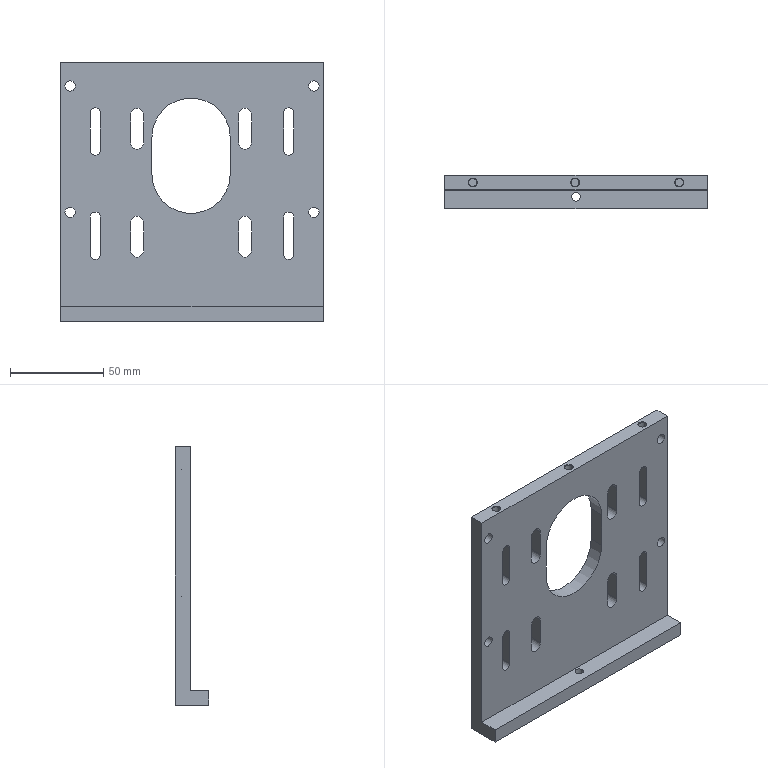Part | STEP file | ROTATION MC_NEW VER-0610_981 | 1 solid | 66 faces | box 141 x 18 x 139 mm | volume 139534 mm3 | plane 33 | cylinder 30 | cone 3 | commonest cylinder face diameters 5.5 x12 7 x8 9 x4 4.2 x3 42 x2 4.5 x1